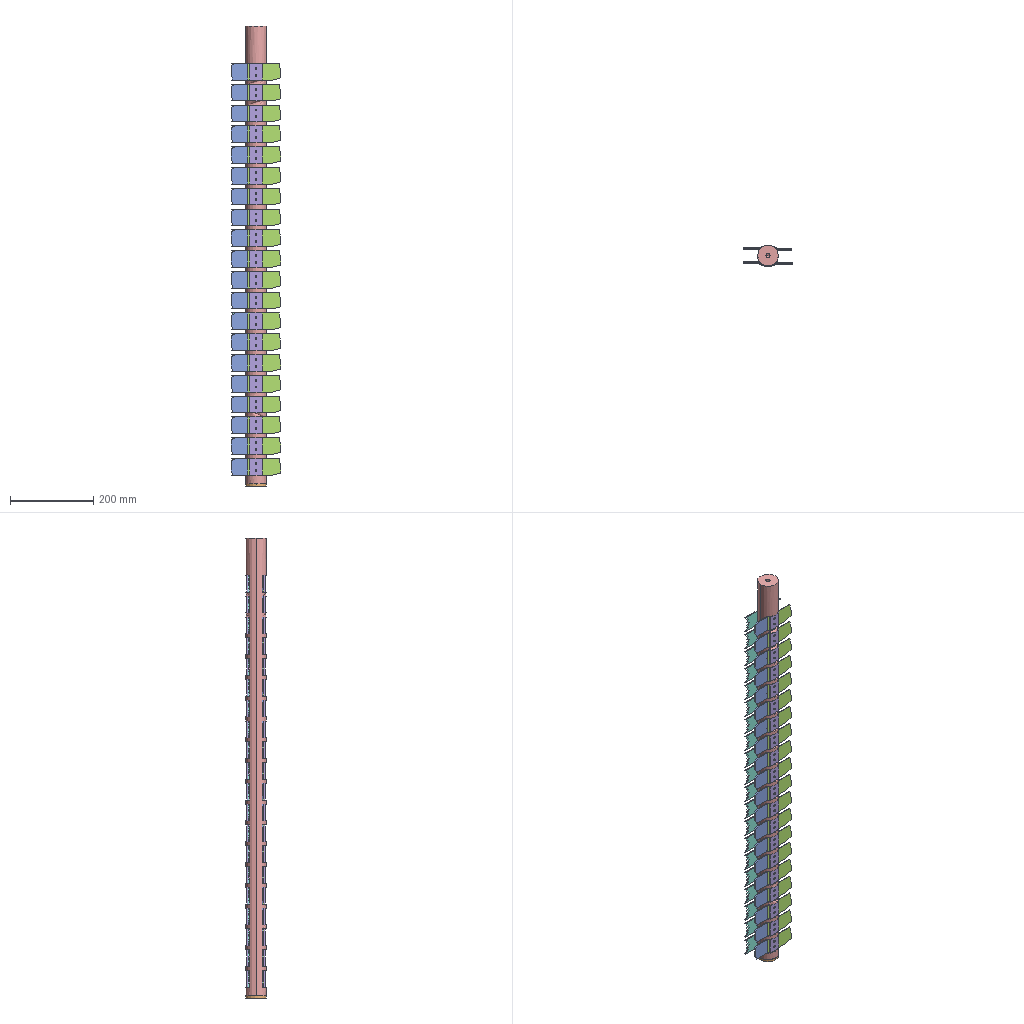Assembly | SolidWorks | 7 different items | 122 placed | box 120 x 50 x 1106 mm
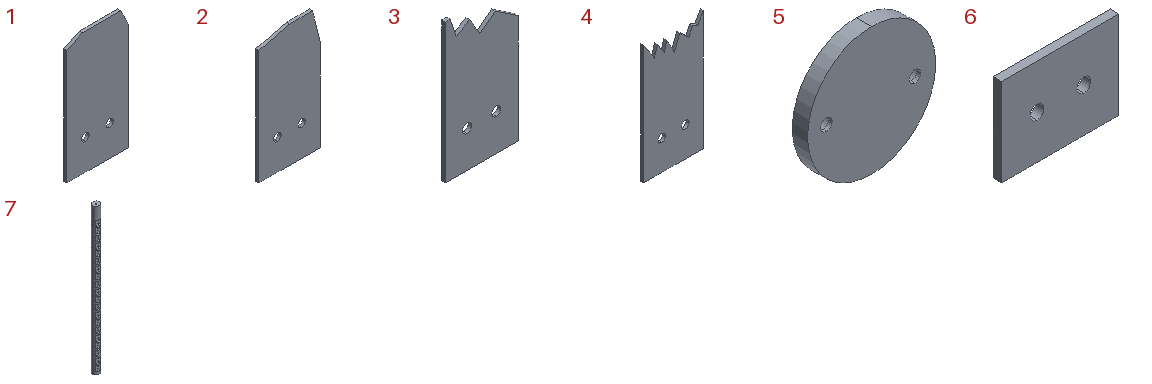Parts list (item | quantity | size | volume | features):
1 | x20 | 40 x 2 x 80 mm | 6221 mm3 | features Chamfer 1, Cut 1, Extrusion 1
2 | x20 | 40 x 2 x 80 mm | 6121 mm3 | features Chamfer 1, Cut 1, Extrusion 1
3 | x20 | 40 x 2 x 76.221 mm | 5242 mm3 | features Cut 2, Extrusion 1
4 | x20 | 40 x 2 x 80 mm | 5747 mm3 | features Cut 2, Extrusion 1
5 | x1 | 50 x 6 x 50 mm | 11274 mm3 | features 3DProfileFeature 1, Extrusion 1, HoleWzd 1
6 | x40 | 40 x 3 x 30 mm | 3491 mm3 | features 3DProfileFeature 1, Extrusion 1, HoleWzd 1
7 | x1 | 50 x 50 x 1100 mm | 1552462 mm3 | features 3DProfileFeature 3, HoleWzd 3, ICE 2, Extrusion 1, LPattern 1, MirrorPattern 1
Mates (type | each side: item.copy, entity, surface, feature):
Coincident | 7.1 face plane Cut-Extrude2 | 1.1 face plane Boss-Extrude1 | 2 times
Coincident | 7.1 edge | 1.1 edge
Concentric | 7.1 face cylinder M4 Tapped Hole1 | 2.1 face cylinder Cut-Extrude1
Coincident | 1.1 face plane Boss-Extrude1 | 2.1 face plane Boss-Extrude1
Parallel | 7.1 face plane LPattern1 | 2.1 face plane Boss-Extrude1
Concentric | 7.1 face cylinder Mirror1 | 3.1 face cylinder Cut-Extrude1 | 2 times
Concentric | 3.1 face cylinder Cut-Extrude1 | 4.1 face cylinder Cut-Extrude1 | 2 times
Coincident | 7.1 face plane Mirror1 | 3.1 face plane Boss-Extrude1
Coincident | 3.1 face plane Boss-Extrude1 | 4.1 face plane Boss-Extrude1
Concentric | 7.1 face cylinder Boss-Extrude1 | 5.1 face cylinder Boss-Extrude1
Coincident | 7.1 face plane Boss-Extrude1 | 5.1 face plane Boss-Extrude1
Coincident | 2.1 face plane Boss-Extrude1 | 6.1 face plane Boss-Extrude1
Coincident | 7.1 face plane Cut-Extrude2 | 6.1 face plane Boss-Extrude1